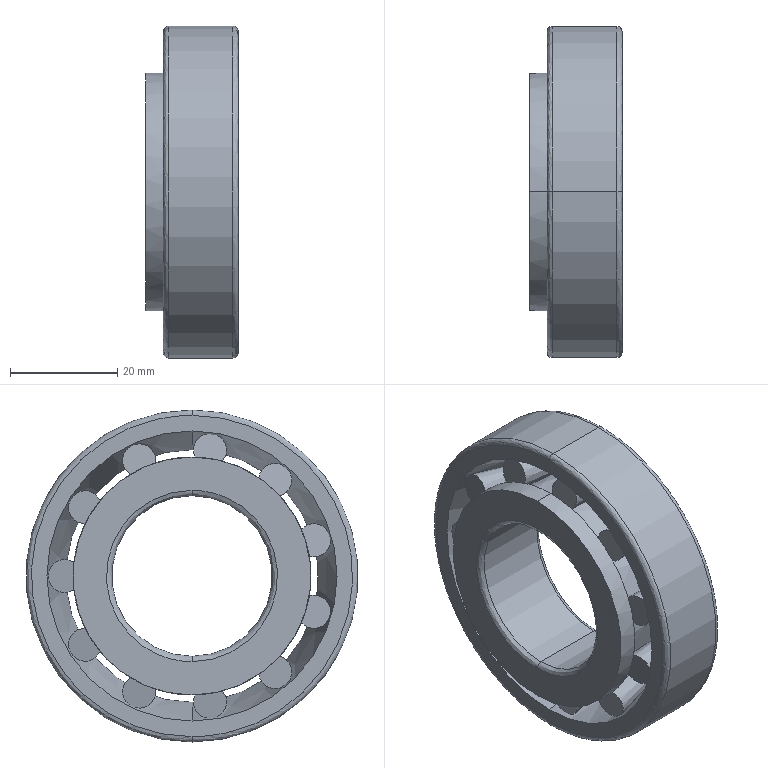Part | SolidWorks | features BaseBody 2 | 2 solids | 72 faces | box 17.25 x 62 x 62 mm | volume 26692 mm3 | cone 30 | plane 26 | spline 8 | cylinder 8 | commonest cylinder face diameters 30 x2 40.806 x2 44.445 x2 62 x2